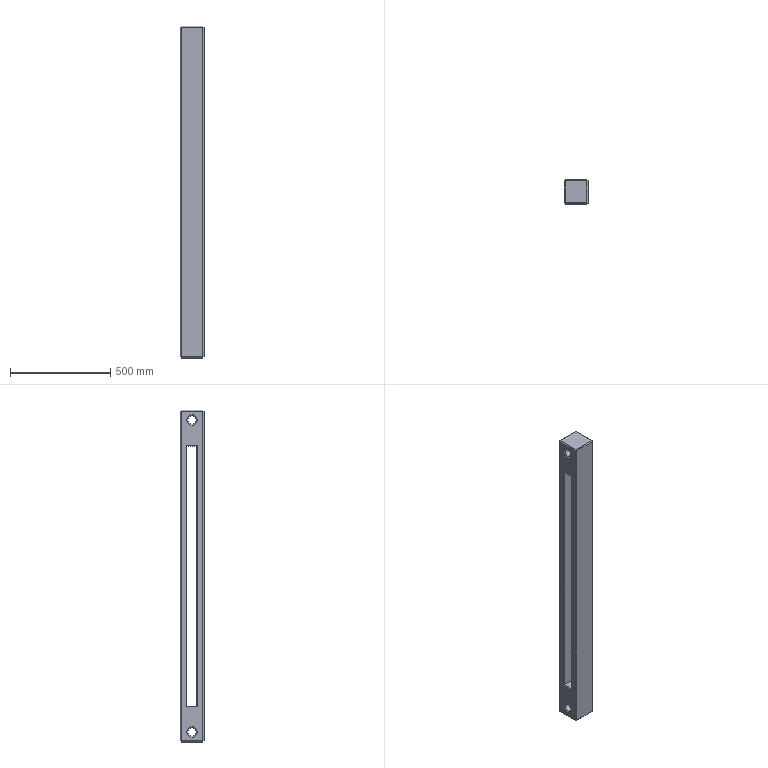Part | SolidWorks | features ICE 2, Chamfer 1, Extrusion 1 | 1 solid | 50 faces | box 120 x 120 x 1660 mm | volume 15602206 mm3 | plane 38 | cone 8 | cylinder 4 | commonest cylinder face diameters 42 x4
STEP:
#1=CARTESIAN_POINT('',(115.,0.,801.));
#2=VERTEX_POINT('',#1);
#3=CARTESIAN_POINT('',(115.,0.,759.));
#4=VERTEX_POINT('',#3);
#5=CARTESIAN_POINT('',(115.,0.,780.));
#6=DIRECTION('',(1.,0.,0.));
#7=DIRECTION('',(0.,0.,-1.));
#8=AXIS2_PLACEMENT_3D('',#5,#6,#7);
#9=CIRCLE('',#8,21.);
#10=EDGE_CURVE('',#2,#4,#9,.T.);
#11=ORIENTED_EDGE('',*,*,#10,.F.);
#12=CARTESIAN_POINT('',(120.,0.,806.));
#13=VERTEX_POINT('',#12);
#14=CARTESIAN_POINT('',(115.,0.,801.));
#15=DIRECTION('',(0.7071,0.,0.7071));
#16=VECTOR('',#15,1000.);
#17=LINE('',#14,#16);
#18=EDGE_CURVE('',#2,#13,#17,.T.);
#19=ORIENTED_EDGE('',*,*,#18,.T.);
#20=CARTESIAN_POINT('',(120.,0.,754.));
#21=VERTEX_POINT('',#20);
#22=CARTESIAN_POINT('',(120.,0.,780.));
#23=DIRECTION('',(-1.,0.,0.));
#24=DIRECTION('',(0.,0.,-1.));
#25=AXIS2_PLACEMENT_3D('',#22,#23,#24);
#26=CIRCLE('',#25,26.);
#27=EDGE_CURVE('',#21,#13,#26,.T.);
#28=ORIENTED_EDGE('',*,*,#27,.F.);
#29=CARTESIAN_POINT('',(115.,0.,759.));
#30=DIRECTION('',(0.7071,0.,-0.7071));
#31=VECTOR('',#30,1000.);
#32=LINE('',#29,#31);
#33=EDGE_CURVE('',#4,#21,#32,.T.);
#34=ORIENTED_EDGE('',*,*,#33,.F.);
#35=EDGE_LOOP('',(#11,#19,#28,#34));
#36=FACE_OUTER_BOUND('',#35,.T.);
#37=CARTESIAN_POINT('',(115.,0.,780.));
#38=DIRECTION('',(1.,0.,0.));
#39=DIRECTION('',(0.,0.,-1.));
#40=AXIS2_PLACEMENT_3D('',#37,#38,#39);
#41=CONICAL_SURFACE('',#40,21.,0.7854);
#42=ADVANCED_FACE('',(#36),#41,.F.);
#43=CARTESIAN_POINT('',(115.,0.,-759.));
#44=VERTEX_POINT('',#43);
#45=CARTESIAN_POINT('',(115.,0.,-801.));
#46=VERTEX_POINT('',#45);
#47=CARTESIAN_POINT('',(115.,0.,-780.));
#48=DIRECTION('',(1.,0.,0.));
#49=DIRECTION('',(0.,0.,-1.));
#50=AXIS2_PLACEMENT_3D('',#47,#48,#49);
#51=CIRCLE('',#50,21.);
#52=EDGE_CURVE('',#44,#46,#51,.T.);
#53=ORIENTED_EDGE('',*,*,#52,.F.);
#54=CARTESIAN_POINT('',(120.,0.,-754.));
#55=VERTEX_POINT('',#54);
#56=CARTESIAN_POINT('',(115.,0.,-759.));
#57=DIRECTION('',(0.7071,0.,0.7071));
#58=VECTOR('',#57,1000.);
#59=LINE('',#56,#58);
#60=EDGE_CURVE('',#44,#55,#59,.T.);
#61=ORIENTED_EDGE('',*,*,#60,.T.);
#62=CARTESIAN_POINT('',(120.,0.,-806.));
#63=VERTEX_POINT('',#62);
#64=CARTESIAN_POINT('',(120.,0.,-780.));
#65=DIRECTION('',(-1.,0.,0.));
#66=DIRECTION('',(0.,0.,-1.));
#67=AXIS2_PLACEMENT_3D('',#64,#65,#66);
#68=CIRCLE('',#67,26.);
#69=EDGE_CURVE('',#63,#55,#68,.T.);
#70=ORIENTED_EDGE('',*,*,#69,.F.);
#71=CARTESIAN_POINT('',(115.,0.,-801.));
#72=DIRECTION('',(0.7071,0.,-0.7071));
#73=VECTOR('',#72,1000.);
#74=LINE('',#71,#73);
#75=EDGE_CURVE('',#46,#63,#74,.T.);
#76=ORIENTED_EDGE('',*,*,#75,.F.);
#77=EDGE_LOOP('',(#53,#61,#70,#76));
#78=FACE_OUTER_BOUND('',#77,.T.);
#79=CARTESIAN_POINT('',(115.,0.,-780.));
#80=DIRECTION('',(1.,0.,0.));
#81=DIRECTION('',(0.,0.,-1.));
#82=AXIS2_PLACEMENT_3D('',#79,#80,#81);
#83=CONICAL_SURFACE('',#82,21.,0.7854);
#84=ADVANCED_FACE('',(#78),#83,.F.);
#85=CARTESIAN_POINT('',(5.,0.,759.));
#86=VERTEX_POINT('',#85);
#87=CARTESIAN_POINT('',(5.,0.,801.));
#88=VERTEX_POINT('',#87);
#89=CARTESIAN_POINT('',(5.,0.,780.));
#90=DIRECTION('',(-1.,0.,0.));
#91=DIRECTION('',(0.,0.,-1.));
#92=AXIS2_PLACEMENT_3D('',#89,#90,#91);
#93=CIRCLE('',#92,21.);
#94=EDGE_CURVE('',#86,#88,#93,.T.);
#95=ORIENTED_EDGE('',*,*,#94,.F.);
#96=CARTESIAN_POINT('',(0.,0.,754.));
#97=VERTEX_POINT('',#96);
#98=CARTESIAN_POINT('',(0.,0.,754.));
#99=DIRECTION('',(-0.7071,0.,-0.7071));
#100=VECTOR('',#99,1000.);
#101=LINE('',#98,#100);
#102=EDGE_CURVE('',#86,#97,#101,.T.);
#103=ORIENTED_EDGE('',*,*,#102,.T.);
#104=CARTESIAN_POINT('',(0.,0.,806.));
#105=VERTEX_POINT('',#104);
#106=CARTESIAN_POINT('',(0.,0.,780.));
#107=DIRECTION('',(1.,0.,0.));
#108=DIRECTION('',(0.,0.,-1.));
#109=AXIS2_PLACEMENT_3D('',#106,#107,#108);
#110=CIRCLE('',#109,26.);
#111=EDGE_CURVE('',#105,#97,#110,.T.);
#112=ORIENTED_EDGE('',*,*,#111,.F.);
#113=CARTESIAN_POINT('',(0.,0.,806.));
#114=DIRECTION('',(-0.7071,0.,0.7071));
#115=VECTOR('',#114,1000.);
#116=LINE('',#113,#115);
#117=EDGE_CURVE('',#88,#105,#116,.T.);
#118=ORIENTED_EDGE('',*,*,#117,.F.);
#119=EDGE_LOOP('',(#95,#103,#112,#118));
#120=FACE_OUTER_BOUND('',#119,.T.);
#121=CARTESIAN_POINT('',(0.,0.,780.));
#122=DIRECTION('',(-1.,0.,0.));
#123=DIRECTION('',(0.,0.,1.));
#124=AXIS2_PLACEMENT_3D('',#121,#122,#123);
#125=CONICAL_SURFACE('',#124,26.,0.7854);
#126=ADVANCED_FACE('',(#120),#125,.F.);
#127=CARTESIAN_POINT('',(5.,0.,-801.));
#128=VERTEX_POINT('',#127);
#129=CARTESIAN_POINT('',(5.,0.,-759.));
#130=VERTEX_POINT('',#129);
#131=CARTESIAN_POINT('',(5.,0.,-780.));
#132=DIRECTION('',(-1.,0.,0.));
#133=DIRECTION('',(0.,0.,-1.));
#134=AXIS2_PLACEMENT_3D('',#131,#132,#133);
#135=CIRCLE('',#134,21.);
#136=EDGE_CURVE('',#128,#130,#135,.T.);
#137=ORIENTED_EDGE('',*,*,#136,.F.);
#138=CARTESIAN_POINT('',(0.,0.,-806.));
#139=VERTEX_POINT('',#138);
#140=CARTESIAN_POINT('',(0.,0.,-806.));
#141=DIRECTION('',(-0.7071,0.,-0.7071));
#142=VECTOR('',#141,1000.);
#143=LINE('',#140,#142);
#144=EDGE_CURVE('',#128,#139,#143,.T.);
#145=ORIENTED_EDGE('',*,*,#144,.T.);
#146=CARTESIAN_POINT('',(0.,0.,-754.));
#147=VERTEX_POINT('',#146);
#148=CARTESIAN_POINT('',(0.,0.,-780.));
#149=DIRECTION('',(1.,0.,0.));
#150=DIRECTION('',(0.,0.,-1.));
#151=AXIS2_PLACEMENT_3D('',#148,#149,#150);
#152=CIRCLE('',#151,26.);
#153=EDGE_CURVE('',#147,#139,#152,.T.);
#154=ORIENTED_EDGE('',*,*,#153,.F.);
#155=CARTESIAN_POINT('',(0.,0.,-754.));
#156=DIRECTION('',(-0.7071,0.,0.7071));
#157=VECTOR('',#156,1000.);
#158=LINE('',#155,#157);
#159=EDGE_CURVE('',#130,#147,#158,.T.);
#160=ORIENTED_EDGE('',*,*,#159,.F.);
#161=EDGE_LOOP('',(#137,#145,#154,#160));
#162=FACE_OUTER_BOUND('',#161,.T.);
#163=CARTESIAN_POINT('',(0.,0.,-780.));
#164=DIRECTION('',(-1.,0.,0.));
#165=DIRECTION('',(0.,0.,1.));
#166=AXIS2_PLACEMENT_3D('',#163,#164,#165);
#167=CONICAL_SURFACE('',#166,26.,0.7854);
#168=ADVANCED_FACE('',(#162),#167,.F.);
#169=ORIENTED_EDGE('',*,*,#94,.T.);
#170=CARTESIAN_POINT('',(0.,0.,801.));
#171=DIRECTION('',(1.,0.,0.));
#172=VECTOR('',#171,1000.);
#173=LINE('',#170,#172);
#174=EDGE_CURVE('',#88,#2,#173,.T.);
#175=ORIENTED_EDGE('',*,*,#174,.T.);
#176=ORIENTED_EDGE('',*,*,#10,.T.);
#177=CARTESIAN_POINT('',(0.,0.,759.));
#178=DIRECTION('',(1.,0.,0.));
#179=VECTOR('',#178,1000.);
#180=LINE('',#177,#179);
#181=EDGE_CURVE('',#86,#4,#180,.T.);
#182=ORIENTED_EDGE('',*,*,#181,.F.);
#183=EDGE_LOOP('',(#169,#175,#176,#182));
#184=FACE_OUTER_BOUND('',#183,.T.);
#185=CARTESIAN_POINT('',(0.,0.,780.));
#186=DIRECTION('',(1.,0.,0.));
#187=DIRECTION('',(0.,0.,-1.));
#188=AXIS2_PLACEMENT_3D('',#185,#186,#187);
#189=CYLINDRICAL_SURFACE('',#188,21.);
#190=ADVANCED_FACE('',(#184),#189,.F.);
#191=ORIENTED_EDGE('',*,*,#136,.T.);
#192=CARTESIAN_POINT('',(0.,0.,-759.));
#193=DIRECTION('',(1.,0.,0.));
#194=VECTOR('',#193,1000.);
#195=LINE('',#192,#194);
#196=EDGE_CURVE('',#130,#44,#195,.T.);
#197=ORIENTED_EDGE('',*,*,#196,.T.);
#198=ORIENTED_EDGE('',*,*,#52,.T.);
#199=CARTESIAN_POINT('',(0.,0.,-801.));
#200=DIRECTION('',(1.,0.,0.));
#201=VECTOR('',#200,1000.);
#202=LINE('',#199,#201);
#203=EDGE_CURVE('',#128,#46,#202,.T.);
#204=ORIENTED_EDGE('',*,*,#203,.F.);
#205=EDGE_LOOP('',(#191,#197,#198,#204));
#206=FACE_OUTER_BOUND('',#205,.T.);
#207=CARTESIAN_POINT('',(0.,0.,-780.));
#208=DIRECTION('',(1.,0.,0.));
#209=DIRECTION('',(0.,0.,-1.));
#210=AXIS2_PLACEMENT_3D('',#207,#208,#209);
#211=CYLINDRICAL_SURFACE('',#210,21.);
#212=ADVANCED_FACE('',(#206),#211,.F.);
#213=CARTESIAN_POINT('',(115.,55.,-830.));
#214=VERTEX_POINT('',#213);
#215=CARTESIAN_POINT('',(115.,-55.,-830.));
#216=VERTEX_POINT('',#215);
#217=CARTESIAN_POINT('',(115.,-60.,-830.));
#218=DIRECTION('',(0.,-1.,0.));
#219=VECTOR('',#218,1000.);
#220=LINE('',#217,#219);
#221=EDGE_CURVE('',#214,#216,#220,.T.);
#222=ORIENTED_EDGE('',*,*,#221,.T.);
#223=CARTESIAN_POINT('',(5.,-55.,-830.));
#224=VERTEX_POINT('',#223);
#225=CARTESIAN_POINT('',(120.,-55.,-830.));
#226=DIRECTION('',(-1.,0.,0.));
#227=VECTOR('',#226,1000.);
#228=LINE('',#225,#227);
#229=EDGE_CURVE('',#216,#224,#228,.T.);
#230=ORIENTED_EDGE('',*,*,#229,.T.);
#231=CARTESIAN_POINT('',(5.,55.,-830.));
#232=VERTEX_POINT('',#231);
#233=CARTESIAN_POINT('',(5.,60.,-830.));
#234=DIRECTION('',(0.,1.,0.));
#235=VECTOR('',#234,1000.);
#236=LINE('',#233,#235);
#237=EDGE_CURVE('',#224,#232,#236,.T.);
#238=ORIENTED_EDGE('',*,*,#237,.T.);
#239=CARTESIAN_POINT('',(120.,55.,-830.));
#240=DIRECTION('',(1.,0.,0.));
#241=VECTOR('',#240,1000.);
#242=LINE('',#239,#241);
#243=EDGE_CURVE('',#232,#214,#242,.T.);
#244=ORIENTED_EDGE('',*,*,#243,.T.);
#245=EDGE_LOOP('',(#222,#230,#238,#244));
#246=FACE_OUTER_BOUND('',#245,.T.);
#247=CARTESIAN_POINT('',(120.,60.,-830.));
#248=DIRECTION('',(0.,0.,1.));
#249=DIRECTION('',(1.,0.,0.));
#250=AXIS2_PLACEMENT_3D('',#247,#248,#249);
#251=PLANE('',#250);
#252=ADVANCED_FACE('',(#246),#251,.F.);
#253=CARTESIAN_POINT('',(115.,60.,-825.));
#254=VERTEX_POINT('',#253);
#255=CARTESIAN_POINT('',(5.,60.,-825.));
#256=VERTEX_POINT('',#255);
#257=CARTESIAN_POINT('',(120.,60.,-825.));
#258=DIRECTION('',(-1.,0.,0.));
#259=VECTOR('',#258,1000.);
#260=LINE('',#257,#259);
#261=EDGE_CURVE('',#254,#256,#260,.T.);
#262=ORIENTED_EDGE('',*,*,#261,.T.);
#263=CARTESIAN_POINT('',(5.,60.,825.));
#264=VERTEX_POINT('',#263);
#265=CARTESIAN_POINT('',(5.,60.,830.));
#266=DIRECTION('',(0.,0.,1.));
#267=VECTOR('',#266,1000.);
#268=LINE('',#265,#267);
#269=EDGE_CURVE('',#256,#264,#268,.T.);
#270=ORIENTED_EDGE('',*,*,#269,.T.);
#271=CARTESIAN_POINT('',(115.,60.,825.));
#272=VERTEX_POINT('',#271);
#273=CARTESIAN_POINT('',(120.,60.,825.));
#274=DIRECTION('',(1.,0.,0.));
#275=VECTOR('',#274,1000.);
#276=LINE('',#273,#275);
#277=EDGE_CURVE('',#264,#272,#276,.T.);
#278=ORIENTED_EDGE('',*,*,#277,.T.);
#279=CARTESIAN_POINT('',(115.,60.,-830.));
#280=DIRECTION('',(0.,0.,-1.));
#281=VECTOR('',#280,1000.);
#282=LINE('',#279,#281);
#283=EDGE_CURVE('',#272,#254,#282,.T.);
#284=ORIENTED_EDGE('',*,*,#283,.T.);
#285=EDGE_LOOP('',(#262,#270,#278,#284));
#286=FACE_OUTER_BOUND('',#285,.T.);
#287=CARTESIAN_POINT('',(120.,60.,830.));
#288=DIRECTION('',(0.,-1.,0.));
#289=DIRECTION('',(0.,0.,-1.));
#290=AXIS2_PLACEMENT_3D('',#287,#288,#289);
#291=PLANE('',#290);
#292=ADVANCED_FACE('',(#286),#291,.F.);
#293=CARTESIAN_POINT('',(115.,-55.,830.));
#294=VERTEX_POINT('',#293);
#295=CARTESIAN_POINT('',(115.,55.,830.));
#296=VERTEX_POINT('',#295);
#297=CARTESIAN_POINT('',(115.,60.,830.));
#298=DIRECTION('',(0.,1.,0.));
#299=VECTOR('',#298,1000.);
#300=LINE('',#297,#299);
#301=EDGE_CURVE('',#294,#296,#300,.T.);
#302=ORIENTED_EDGE('',*,*,#301,.T.);
#303=CARTESIAN_POINT('',(5.,55.,830.));
#304=VERTEX_POINT('',#303);
#305=CARTESIAN_POINT('',(120.,55.,830.));
#306=DIRECTION('',(-1.,0.,0.));
#307=VECTOR('',#306,1000.);
#308=LINE('',#305,#307);
#309=EDGE_CURVE('',#296,#304,#308,.T.);
#310=ORIENTED_EDGE('',*,*,#309,.T.);
#311=CARTESIAN_POINT('',(5.,-55.,830.));
#312=VERTEX_POINT('',#311);
#313=CARTESIAN_POINT('',(5.,60.,830.));
#314=DIRECTION('',(0.,-1.,0.));
#315=VECTOR('',#314,1000.);
#316=LINE('',#313,#315);
#317=EDGE_CURVE('',#304,#312,#316,.T.);
#318=ORIENTED_EDGE('',*,*,#317,.T.);
#319=CARTESIAN_POINT('',(120.,-55.,830.));
#320=DIRECTION('',(1.,0.,0.));
#321=VECTOR('',#320,1000.);
#322=LINE('',#319,#321);
#323=EDGE_CURVE('',#312,#294,#322,.T.);
#324=ORIENTED_EDGE('',*,*,#323,.T.);
#325=EDGE_LOOP('',(#302,#310,#318,#324));
#326=FACE_OUTER_BOUND('',#325,.T.);
#327=CARTESIAN_POINT('',(120.,60.,830.));
#328=DIRECTION('',(0.,0.,-1.));
#329=DIRECTION('',(-1.,0.,0.));
#330=AXIS2_PLACEMENT_3D('',#327,#328,#329);
#331=PLANE('',#330);
#332=ADVANCED_FACE('',(#326),#331,.F.);
#333=CARTESIAN_POINT('',(115.,-60.,825.));
#334=VERTEX_POINT('',#333);
#335=CARTESIAN_POINT('',(5.,-60.,825.));
#336=VERTEX_POINT('',#335);
#337=CARTESIAN_POINT('',(120.,-60.,825.));
#338=DIRECTION('',(-1.,0.,0.));
#339=VECTOR('',#338,1000.);
#340=LINE('',#337,#339);
#341=EDGE_CURVE('',#334,#336,#340,.T.);
#342=ORIENTED_EDGE('',*,*,#341,.T.);
#343=CARTESIAN_POINT('',(5.,-60.,-825.));
#344=VERTEX_POINT('',#343);
#345=CARTESIAN_POINT('',(5.,-60.,830.));
#346=DIRECTION('',(0.,0.,-1.));
#347=VECTOR('',#346,1000.);
#348=LINE('',#345,#347);
#349=EDGE_CURVE('',#336,#344,#348,.T.);
#350=ORIENTED_EDGE('',*,*,#349,.T.);
#351=CARTESIAN_POINT('',(115.,-60.,-825.));
#352=VERTEX_POINT('',#351);
#353=CARTESIAN_POINT('',(120.,-60.,-825.));
#354=DIRECTION('',(1.,0.,0.));
#355=VECTOR('',#354,1000.);
#356=LINE('',#353,#355);
#357=EDGE_CURVE('',#344,#352,#356,.T.);
#358=ORIENTED_EDGE('',*,*,#357,.T.);
#359=CARTESIAN_POINT('',(115.,-60.,830.));
#360=DIRECTION('',(0.,0.,1.));
#361=VECTOR('',#360,1000.);
#362=LINE('',#359,#361);
#363=EDGE_CURVE('',#352,#334,#362,.T.);
#364=ORIENTED_EDGE('',*,*,#363,.T.);
#365=EDGE_LOOP('',(#342,#350,#358,#364));
#366=FACE_OUTER_BOUND('',#365,.T.);
#367=CARTESIAN_POINT('',(120.,-60.,830.));
#368=DIRECTION('',(0.,1.,0.));
#369=DIRECTION('',(0.,0.,1.));
#370=AXIS2_PLACEMENT_3D('',#367,#368,#369);
#371=PLANE('',#370);
#372=ADVANCED_FACE('',(#366),#371,.F.);
#373=CARTESIAN_POINT('',(120.,-30.,655.));
#374=VERTEX_POINT('',#373);
#375=CARTESIAN_POINT('',(120.,30.,655.));
#376=VERTEX_POINT('',#375);
#377=CARTESIAN_POINT('',(120.,25.,655.));
#378=DIRECTION('',(0.,1.,0.));
#379=VECTOR('',#378,1000.);
#380=LINE('',#377,#379);
#381=EDGE_CURVE('',#374,#376,#380,.T.);
#382=ORIENTED_EDGE('',*,*,#381,.T.);
#383=CARTESIAN_POINT('',(120.,30.,-655.));
#384=VERTEX_POINT('',#383);
#385=CARTESIAN_POINT('',(120.,30.,-650.));
#386=DIRECTION('',(0.,0.,-1.));
#387=VECTOR('',#386,1000.);
#388=LINE('',#385,#387);
#389=EDGE_CURVE('',#376,#384,#388,.T.);
#390=ORIENTED_EDGE('',*,*,#389,.T.);
#391=CARTESIAN_POINT('',(120.,-30.,-655.));
#392=VERTEX_POINT('',#391);
#393=CARTESIAN_POINT('',(120.,-25.,-655.));
#394=DIRECTION('',(0.,-1.,0.));
#395=VECTOR('',#394,1000.);
#396=LINE('',#393,#395);
#397=EDGE_CURVE('',#384,#392,#396,.T.);
#398=ORIENTED_EDGE('',*,*,#397,.T.);
#399=CARTESIAN_POINT('',(120.,-30.,650.));
#400=DIRECTION('',(0.,0.,1.));
#401=VECTOR('',#400,1000.);
#402=LINE('',#399,#401);
#403=EDGE_CURVE('',#392,#374,#402,.T.);
#404=ORIENTED_EDGE('',*,*,#403,.T.);
#405=EDGE_LOOP('',(#382,#390,#398,#404));
#406=FACE_BOUND('',#405,.T.);
#407=ORIENTED_EDGE('',*,*,#69,.T.);
#408=CARTESIAN_POINT('',(120.,0.,-780.));
#409=DIRECTION('',(-1.,0.,0.));
#410=DIRECTION('',(0.,0.,-1.));
#411=AXIS2_PLACEMENT_3D('',#408,#409,#410);
#412=CIRCLE('',#411,26.);
#413=EDGE_CURVE('',#55,#63,#412,.T.);
#414=ORIENTED_EDGE('',*,*,#413,.T.);
#415=EDGE_LOOP('',(#407,#414));
#416=FACE_BOUND('',#415,.T.);
#417=ORIENTED_EDGE('',*,*,#27,.T.);
#418=CARTESIAN_POINT('',(120.,0.,780.));
#419=DIRECTION('',(-1.,0.,0.));
#420=DIRECTION('',(0.,0.,-1.));
#421=AXIS2_PLACEMENT_3D('',#418,#419,#420);
#422=CIRCLE('',#421,26.);
#423=EDGE_CURVE('',#13,#21,#422,.T.);
#424=ORIENTED_EDGE('',*,*,#423,.T.);
#425=EDGE_LOOP('',(#417,#424));
#426=FACE_BOUND('',#425,.T.);
#427=CARTESIAN_POINT('',(120.,55.,825.));
#428=VERTEX_POINT('',#427);
#429=CARTESIAN_POINT('',(120.,-55.,825.));
#430=VERTEX_POINT('',#429);
#431=CARTESIAN_POINT('',(120.,-60.,825.));
#432=DIRECTION('',(0.,-1.,0.));
#433=VECTOR('',#432,1000.);
#434=LINE('',#431,#433);
#435=EDGE_CURVE('',#428,#430,#434,.T.);
#436=ORIENTED_EDGE('',*,*,#435,.T.);
#437=CARTESIAN_POINT('',(120.,-55.,-825.));
#438=VERTEX_POINT('',#437);
#439=CARTESIAN_POINT('',(120.,-55.,-830.));
#440=DIRECTION('',(0.,0.,-1.));
#441=VECTOR('',#440,1000.);
#442=LINE('',#439,#441);
#443=EDGE_CURVE('',#430,#438,#442,.T.);
#444=ORIENTED_EDGE('',*,*,#443,.T.);
#445=CARTESIAN_POINT('',(120.,55.,-825.));
#446=VERTEX_POINT('',#445);
#447=CARTESIAN_POINT('',(120.,60.,-825.));
#448=DIRECTION('',(0.,1.,0.));
#449=VECTOR('',#448,1000.);
#450=LINE('',#447,#449);
#451=EDGE_CURVE('',#438,#446,#450,.T.);
#452=ORIENTED_EDGE('',*,*,#451,.T.);
#453=CARTESIAN_POINT('',(120.,55.,830.));
#454=DIRECTION('',(0.,0.,1.));
#455=VECTOR('',#454,1000.);
#456=LINE('',#453,#455);
#457=EDGE_CURVE('',#446,#428,#456,.T.);
#458=ORIENTED_EDGE('',*,*,#457,.T.);
#459=EDGE_LOOP('',(#436,#444,#452,#458));
#460=FACE_OUTER_BOUND('',#459,.T.);
#461=CARTESIAN_POINT('',(120.,0.,0.));
#462=DIRECTION('',(1.,0.,0.));
#463=DIRECTION('',(0.,0.,-1.));
#464=AXIS2_PLACEMENT_3D('',#461,#462,#463);
#465=PLANE('',#464);
#466=ADVANCED_FACE('',(#406,#416,#426,#460),#465,.T.);
#467=CARTESIAN_POINT('',(0.,30.,-655.));
#468=VERTEX_POINT('',#467);
#469=CARTESIAN_POINT('',(0.,30.,655.));
#470=VERTEX_POINT('',#469);
#471=CARTESIAN_POINT('',(0.,30.,0.));
#472=DIRECTION('',(0.,0.,1.));
#473=VECTOR('',#472,1000.);
#474=LINE('',#471,#473);
#475=EDGE_CURVE('',#468,#470,#474,.T.);
#476=ORIENTED_EDGE('',*,*,#475,.T.);
#477=CARTESIAN_POINT('',(0.,-30.,655.));
#478=VERTEX_POINT('',#477);
#479=CARTESIAN_POINT('',(0.,0.,655.));
#480=DIRECTION('',(0.,-1.,0.));
#481=VECTOR('',#480,1000.);
#482=LINE('',#479,#481);
#483=EDGE_CURVE('',#470,#478,#482,.T.);
#484=ORIENTED_EDGE('',*,*,#483,.T.);
#485=CARTESIAN_POINT('',(0.,-30.,-655.));
#486=VERTEX_POINT('',#485);
#487=CARTESIAN_POINT('',(0.,-30.,0.));
#488=DIRECTION('',(0.,0.,-1.));
#489=VECTOR('',#488,1000.);
#490=LINE('',#487,#489);
#491=EDGE_CURVE('',#478,#486,#490,.T.);
#492=ORIENTED_EDGE('',*,*,#491,.T.);
#493=CARTESIAN_POINT('',(0.,0.,-655.));
#494=DIRECTION('',(0.,1.,0.));
#495=VECTOR('',#494,1000.);
#496=LINE('',#493,#495);
#497=EDGE_CURVE('',#486,#468,#496,.T.);
#498=ORIENTED_EDGE('',*,*,#497,.T.);
#499=EDGE_LOOP('',(#476,#484,#492,#498));
#500=FACE_BOUND('',#499,.T.);
#501=ORIENTED_EDGE('',*,*,#153,.T.);
#502=CARTESIAN_POINT('',(0.,0.,-780.));
#503=DIRECTION('',(1.,0.,0.));
#504=DIRECTION('',(0.,0.,-1.));
#505=AXIS2_PLACEMENT_3D('',#502,#503,#504);
#506=CIRCLE('',#505,26.);
#507=EDGE_CURVE('',#139,#147,#506,.T.);
#508=ORIENTED_EDGE('',*,*,#507,.T.);
#509=EDGE_LOOP('',(#501,#508));
#510=FACE_BOUND('',#509,.T.);
#511=ORIENTED_EDGE('',*,*,#111,.T.);
#512=CARTESIAN_POINT('',(0.,0.,780.));
#513=DIRECTION('',(1.,0.,0.));
#514=DIRECTION('',(0.,0.,-1.));
#515=AXIS2_PLACEMENT_3D('',#512,#513,#514);
#516=CIRCLE('',#515,26.);
#517=EDGE_CURVE('',#97,#105,#516,.T.);
#518=ORIENTED_EDGE('',*,*,#517,.T.);
#519=EDGE_LOOP('',(#511,#518));
#520=FACE_BOUND('',#519,.T.);
#521=CARTESIAN_POINT('',(0.,55.,825.));
#522=VERTEX_POINT('',#521);
#523=CARTESIAN_POINT('',(0.,55.,-825.));
#524=VERTEX_POINT('',#523);
#525=CARTESIAN_POINT('',(0.,55.,0.));
#526=DIRECTION('',(0.,0.,-1.));
#527=VECTOR('',#526,1000.);
#528=LINE('',#525,#527);
#529=EDGE_CURVE('',#522,#524,#528,.T.);
#530=ORIENTED_EDGE('',*,*,#529,.T.);
#531=CARTESIAN_POINT('',(0.,-55.,-825.));
#532=VERTEX_POINT('',#531);
#533=CARTESIAN_POINT('',(0.,0.,-825.));
#534=DIRECTION('',(0.,-1.,0.));
#535=VECTOR('',#534,1000.);
#536=LINE('',#533,#535);
#537=EDGE_CURVE('',#524,#532,#536,.T.);
#538=ORIENTED_EDGE('',*,*,#537,.T.);
#539=CARTESIAN_POINT('',(0.,-55.,825.));
#540=VERTEX_POINT('',#539);
#541=CARTESIAN_POINT('',(0.,-55.,0.));
#542=DIRECTION('',(0.,0.,1.));
#543=VECTOR('',#542,1000.);
#544=LINE('',#541,#543);
#545=EDGE_CURVE('',#532,#540,#544,.T.);
#546=ORIENTED_EDGE('',*,*,#545,.T.);
#547=CARTESIAN_POINT('',(0.,0.,825.));
#548=DIRECTION('',(0.,1.,0.));
#549=VECTOR('',#548,1000.);
#550=LINE('',#547,#549);
#551=EDGE_CURVE('',#540,#522,#550,.T.);
#552=ORIENTED_EDGE('',*,*,#551,.T.);
#553=EDGE_LOOP('',(#530,#538,#546,#552));
#554=FACE_OUTER_BOUND('',#553,.T.);
#555=CARTESIAN_POINT('',(0.,0.,0.));
#556=DIRECTION('',(1.,0.,0.));
#557=DIRECTION('',(0.,0.,-1.));
#558=AXIS2_PLACEMENT_3D('',#555,#556,#557);
#559=PLANE('',#558);
#560=ADVANCED_FACE('',(#500,#510,#520,#554),#559,.F.);
#561=CARTESIAN_POINT('',(5.,25.,-650.));
#562=VERTEX_POINT('',#561);
#563=CARTESIAN_POINT('',(115.,25.,-650.));
#564=VERTEX_POINT('',#563);
#565=CARTESIAN_POINT('',(0.,25.,-650.));
#566=DIRECTION('',(1.,0.,0.));
#567=VECTOR('',#566,1000.);
#568=LINE('',#565,#567);
#569=EDGE_CURVE('',#562,#564,#568,.T.);
#570=ORIENTED_EDGE('',*,*,#569,.F.);
#571=CARTESIAN_POINT('',(5.,-25.,-650.));
#572=VERTEX_POINT('',#571);
#573=CARTESIAN_POINT('',(5.,25.,-650.));
#574=DIRECTION('',(0.,-1.,0.));
#575=VECTOR('',#574,1000.);
#576=LINE('',#573,#575);
#577=EDGE_CURVE('',#562,#572,#576,.T.);
#578=ORIENTED_EDGE('',*,*,#577,.T.);
#579=CARTESIAN_POINT('',(115.,-25.,-650.));
#580=VERTEX_POINT('',#579);
#581=CARTESIAN_POINT('',(0.,-25.,-650.));
#582=DIRECTION('',(1.,0.,0.));
#583=VECTOR('',#582,1000.);
#584=LINE('',#581,#583);
#585=EDGE_CURVE('',#572,#580,#584,.T.);
#586=ORIENTED_EDGE('',*,*,#585,.T.);
#587=CARTESIAN_POINT('',(115.,25.,-650.));
#588=DIRECTION('',(0.,1.,0.));
#589=VECTOR('',#588,1000.);
#590=LINE('',#587,#589);
#591=EDGE_CURVE('',#580,#564,#590,.T.);
#592=ORIENTED_EDGE('',*,*,#591,.T.);
#593=EDGE_LOOP('',(#570,#578,#586,#592));
#594=FACE_OUTER_BOUND('',#593,.T.);
#595=CARTESIAN_POINT('',(0.,25.,-650.));
#596=DIRECTION('',(0.,0.,-1.));
#597=DIRECTION('',(-1.,0.,0.));
#598=AXIS2_PLACEMENT_3D('',#595,#596,#597);
#599=PLANE('',#598);
#600=ADVANCED_FACE('',(#594),#599,.F.);
#601=ORIENTED_EDGE('',*,*,#585,.F.);
#602=CARTESIAN_POINT('',(5.,-25.,650.));
#603=VERTEX_POINT('',#602);
#604=CARTESIAN_POINT('',(5.,-25.,650.));
#605=DIRECTION('',(0.,0.,1.));
#606=VECTOR('',#605,1000.);
#607=LINE('',#604,#606);
#608=EDGE_CURVE('',#572,#603,#607,.T.);
#609=ORIENTED_EDGE('',*,*,#608,.T.);
#610=CARTESIAN_POINT('',(115.,-25.,650.));
#611=VERTEX_POINT('',#610);
#612=CARTESIAN_POINT('',(0.,-25.,650.));
#613=DIRECTION('',(1.,0.,0.));
#614=VECTOR('',#613,1000.);
#615=LINE('',#612,#614);
#616=EDGE_CURVE('',#603,#611,#615,.T.);
#617=ORIENTED_EDGE('',*,*,#616,.T.);
#618=CARTESIAN_POINT('',(115.,-25.,-650.));
#619=DIRECTION('',(0.,0.,-1.));
#620=VECTOR('',#619,1000.);
#621=LINE('',#618,#620);
#622=EDGE_CURVE('',#611,#580,#621,.T.);
#623=ORIENTED_EDGE('',*,*,#622,.T.);
#624=EDGE_LOOP('',(#601,#609,#617,#623));
#625=FACE_OUTER_BOUND('',#624,.T.);
#626=CARTESIAN_POINT('',(0.,-25.,650.));
#627=DIRECTION('',(0.,-1.,0.));
#628=DIRECTION('',(0.,0.,-1.));
#629=AXIS2_PLACEMENT_3D('',#626,#627,#628);
#630=PLANE('',#629);
#631=ADVANCED_FACE('',(#625),#630,.F.);
#632=ORIENTED_EDGE('',*,*,#616,.F.);
#633=CARTESIAN_POINT('',(5.,25.,650.));
#634=VERTEX_POINT('',#633);
#635=CARTESIAN_POINT('',(5.,25.,650.));
#636=DIRECTION('',(0.,1.,0.));
#637=VECTOR('',#636,1000.);
#638=LINE('',#635,#637);
#639=EDGE_CURVE('',#603,#634,#638,.T.);
#640=ORIENTED_EDGE('',*,*,#639,.T.);
#641=CARTESIAN_POINT('',(115.,25.,650.));
#642=VERTEX_POINT('',#641);
#643=CARTESIAN_POINT('',(0.,25.,650.));
#644=DIRECTION('',(1.,0.,0.));
#645=VECTOR('',#644,1000.);
#646=LINE('',#643,#645);
#647=EDGE_CURVE('',#634,#642,#646,.T.);
#648=ORIENTED_EDGE('',*,*,#647,.T.);
#649=CARTESIAN_POINT('',(115.,-25.,650.));
#650=DIRECTION('',(0.,-1.,0.));
#651=VECTOR('',#650,1000.);
#652=LINE('',#649,#651);
#653=EDGE_CURVE('',#642,#611,#652,.T.);
#654=ORIENTED_EDGE('',*,*,#653,.T.);
#655=EDGE_LOOP('',(#632,#640,#648,#654));
#656=FACE_OUTER_BOUND('',#655,.T.);
#657=CARTESIAN_POINT('',(0.,25.,650.));
#658=DIRECTION('',(0.,0.,1.));
#659=DIRECTION('',(1.,0.,0.));
#660=AXIS2_PLACEMENT_3D('',#657,#658,#659);
#661=PLANE('',#660);
#662=ADVANCED_FACE('',(#656),#661,.F.);
#663=ORIENTED_EDGE('',*,*,#647,.F.);
#664=CARTESIAN_POINT('',(5.,25.,650.));
#665=DIRECTION('',(0.,0.,-1.));
#666=VECTOR('',#665,1000.);
#667=LINE('',#664,#666);
#668=EDGE_CURVE('',#634,#562,#667,.T.);
#669=ORIENTED_EDGE('',*,*,#668,.T.);
#670=ORIENTED_EDGE('',*,*,#569,.T.);
#671=CARTESIAN_POINT('',(115.,25.,650.));
#672=DIRECTION('',(0.,0.,1.));
#673=VECTOR('',#672,1000.);
#674=LINE('',#671,#673);
#675=EDGE_CURVE('',#564,#642,#674,.T.);
#676=ORIENTED_EDGE('',*,*,#675,.T.);
#677=EDGE_LOOP('',(#663,#669,#670,#676));
#678=FACE_OUTER_BOUND('',#677,.T.);
#679=CARTESIAN_POINT('',(0.,25.,650.));
#680=DIRECTION('',(0.,1.,0.));
#681=DIRECTION('',(0.,0.,1.));
#682=AXIS2_PLACEMENT_3D('',#679,#680,#681);
#683=PLANE('',#682);
#684=ADVANCED_FACE('',(#678),#683,.F.);
#685=ORIENTED_EDGE('',*,*,#196,.F.);
#686=CARTESIAN_POINT('',(5.,0.,-780.));
#687=DIRECTION('',(-1.,0.,0.));
#688=DIRECTION('',(0.,0.,-1.));
#689=AXIS2_PLACEMENT_3D('',#686,#687,#688);
#690=CIRCLE('',#689,21.);
#691=EDGE_CURVE('',#130,#128,#690,.T.);
#692=ORIENTED_EDGE('',*,*,#691,.T.);
#693=ORIENTED_EDGE('',*,*,#203,.T.);
#694=CARTESIAN_POINT('',(115.,0.,-780.));
#695=DIRECTION('',(1.,0.,0.));
#696=DIRECTION('',(0.,0.,-1.));
#697=AXIS2_PLACEMENT_3D('',#694,#695,#696);
#698=CIRCLE('',#697,21.);
#699=EDGE_CURVE('',#46,#44,#698,.T.);
#700=ORIENTED_EDGE('',*,*,#699,.T.);
#701=EDGE_LOOP('',(#685,#692,#693,#700));
#702=FACE_OUTER_BOUND('',#701,.T.);
#703=CARTESIAN_POINT('',(0.,0.,-780.));
#704=DIRECTION('',(1.,0.,0.));
#705=DIRECTION('',(0.,0.,-1.));
#706=AXIS2_PLACEMENT_3D('',#703,#704,#705);
#707=CYLINDRICAL_SURFACE('',#706,21.);
#708=ADVANCED_FACE('',(#702),#707,.F.);
#709=ORIENTED_EDGE('',*,*,#174,.F.);
#710=CARTESIAN_POINT('',(5.,0.,780.));
#711=DIRECTION('',(-1.,0.,0.));
#712=DIRECTION('',(0.,0.,-1.));
#713=AXIS2_PLACEMENT_3D('',#710,#711,#712);
#714=CIRCLE('',#713,21.);
#715=EDGE_CURVE('',#88,#86,#714,.T.);
#716=ORIENTED_EDGE('',*,*,#715,.T.);
#717=ORIENTED_EDGE('',*,*,#181,.T.);
#718=CARTESIAN_POINT('',(115.,0.,780.));
#719=DIRECTION('',(1.,0.,0.));
#720=DIRECTION('',(0.,0.,-1.));
#721=AXIS2_PLACEMENT_3D('',#718,#719,#720);
#722=CIRCLE('',#721,21.);
#723=EDGE_CURVE('',#4,#2,#722,.T.);
#724=ORIENTED_EDGE('',*,*,#723,.T.);
#725=EDGE_LOOP('',(#709,#716,#717,#724));
#726=FACE_OUTER_BOUND('',#725,.T.);
#727=CARTESIAN_POINT('',(0.,0.,780.));
#728=DIRECTION('',(1.,0.,0.));
#729=DIRECTION('',(0.,0.,-1.));
#730=AXIS2_PLACEMENT_3D('',#727,#728,#729);
#731=CYLINDRICAL_SURFACE('',#730,21.);
#732=ADVANCED_FACE('',(#726),#731,.F.);
#733=CARTESIAN_POINT('',(10.,-20.,-645.));
#734=DIRECTION('',(-0.5774,-0.5774,-0.5774));
#735=VECTOR('',#734,1000.);
#736=LINE('',#733,#735);
#737=EDGE_CURVE('',#572,#486,#736,.T.);
#738=ORIENTED_EDGE('',*,*,#737,.F.);
#739=ORIENTED_EDGE('',*,*,#577,.F.);
#740=CARTESIAN_POINT('',(218.333,-188.333,-436.667));
#741=DIRECTION('',(0.5774,-0.5774,0.5774));
#742=VECTOR('',#741,1000.);
#743=LINE('',#740,#742);
#744=EDGE_CURVE('',#468,#562,#743,.T.);
#745=ORIENTED_EDGE('',*,*,#744,.F.);
#746=ORIENTED_EDGE('',*,*,#497,.F.);
#747=EDGE_LOOP('',(#738,#739,#745,#746));
#748=FACE_OUTER_BOUND('',#747,.T.);
#749=CARTESIAN_POINT('',(0.,0.,-655.));
#750=DIRECTION('',(0.7071,0.,-0.7071));
#751=DIRECTION('',(0.,1.,0.));
#752=AXIS2_PLACEMENT_3D('',#749,#750,#751);
#753=PLANE('',#752);
#754=ADVANCED_FACE('',(#748),#753,.F.);
#755=ORIENTED_EDGE('',*,*,#744,.T.);
#756=ORIENTED_EDGE('',*,*,#668,.F.);
#757=CARTESIAN_POINT('',(10.,20.,645.));
#758=DIRECTION('',(0.5774,-0.5774,-0.5774));
#759=VECTOR('',#758,1000.);
#760=LINE('',#757,#759);
#761=EDGE_CURVE('',#470,#634,#760,.T.);
#762=ORIENTED_EDGE('',*,*,#761,.F.);
#763=ORIENTED_EDGE('',*,*,#475,.F.);
#764=EDGE_LOOP('',(#755,#756,#762,#763));
#765=FACE_OUTER_BOUND('',#764,.T.);
#766=CARTESIAN_POINT('',(0.,30.,0.));
#767=DIRECTION('',(0.7071,0.7071,0.));
#768=DIRECTION('',(0.,0.,1.));
#769=AXIS2_PLACEMENT_3D('',#766,#767,#768);
#770=PLANE('',#769);
#771=ADVANCED_FACE('',(#765),#770,.F.);
#772=ORIENTED_EDGE('',*,*,#737,.T.);
#773=ORIENTED_EDGE('',*,*,#491,.F.);
#774=CARTESIAN_POINT('',(10.,-20.,645.));
#775=DIRECTION('',(-0.5774,-0.5774,0.5774));
#776=VECTOR('',#775,1000.);
#777=LINE('',#774,#776);
#778=EDGE_CURVE('',#603,#478,#777,.T.);
#779=ORIENTED_EDGE('',*,*,#778,.F.);
#780=ORIENTED_EDGE('',*,*,#608,.F.);
#781=EDGE_LOOP('',(#772,#773,#779,#780));
#782=FACE_OUTER_BOUND('',#781,.T.);
#783=CARTESIAN_POINT('',(0.,-30.,0.));
#784=DIRECTION('',(0.7071,-0.7071,0.));
#785=DIRECTION('',(0.,0.,-1.));
#786=AXIS2_PLACEMENT_3D('',#783,#784,#785);
#787=PLANE('',#786);
#788=ADVANCED_FACE('',(#782),#787,.F.);
#789=ORIENTED_EDGE('',*,*,#761,.T.);
#790=ORIENTED_EDGE('',*,*,#639,.F.);
#791=ORIENTED_EDGE('',*,*,#778,.T.);
#792=ORIENTED_EDGE('',*,*,#483,.F.);
#793=EDGE_LOOP('',(#789,#790,#791,#792));
#794=FACE_OUTER_BOUND('',#793,.T.);
#795=CARTESIAN_POINT('',(0.,0.,655.));
#796=DIRECTION('',(0.7071,0.,0.7071));
#797=DIRECTION('',(0.,-1.,0.));
#798=AXIS2_PLACEMENT_3D('',#795,#796,#797);
#799=PLANE('',#798);
#800=ADVANCED_FACE('',(#794),#799,.F.);
#801=ORIENTED_EDGE('',*,*,#144,.F.);
#802=ORIENTED_EDGE('',*,*,#691,.F.);
#803=ORIENTED_EDGE('',*,*,#159,.T.);
#804=ORIENTED_EDGE('',*,*,#507,.F.);
#805=EDGE_LOOP('',(#801,#802,#803,#804));
#806=FACE_OUTER_BOUND('',#805,.T.);
#807=CARTESIAN_POINT('',(0.,0.,-780.));
#808=DIRECTION('',(-1.,0.,0.));
#809=DIRECTION('',(0.,0.,1.));
#810=AXIS2_PLACEMENT_3D('',#807,#808,#809);
#811=CONICAL_SURFACE('',#810,26.,0.7854);
#812=ADVANCED_FACE('',(#806),#811,.F.);
#813=ORIENTED_EDGE('',*,*,#102,.F.);
#814=ORIENTED_EDGE('',*,*,#715,.F.);
#815=ORIENTED_EDGE('',*,*,#117,.T.);
#816=ORIENTED_EDGE('',*,*,#517,.F.);
#817=EDGE_LOOP('',(#813,#814,#815,#816));
#818=FACE_OUTER_BOUND('',#817,.T.);
#819=CARTESIAN_POINT('',(0.,0.,780.));
#820=DIRECTION('',(-1.,0.,0.));
#821=DIRECTION('',(0.,0.,1.));
#822=AXIS2_PLACEMENT_3D('',#819,#820,#821);
#823=CONICAL_SURFACE('',#822,26.,0.7854);
#824=ADVANCED_FACE('',(#818),#823,.F.);
#825=CARTESIAN_POINT('',(98.333,-8.333,633.333));
#826=DIRECTION('',(-0.5774,0.5774,-0.5774));
#827=VECTOR('',#826,1000.);
#828=LINE('',#825,#827);
#829=EDGE_CURVE('',#374,#611,#828,.T.);
#830=ORIENTED_EDGE('',*,*,#829,.F.);
#831=ORIENTED_EDGE('',*,*,#403,.F.);
#832=CARTESIAN_POINT('',(-318.333,408.333,-216.667));
#833=DIRECTION('',(0.5774,-0.5774,-0.5774));
#834=VECTOR('',#833,1000.);
#835=LINE('',#832,#834);
#836=EDGE_CURVE('',#580,#392,#835,.T.);
#837=ORIENTED_EDGE('',*,*,#836,.F.);
#838=ORIENTED_EDGE('',*,*,#622,.F.);
#839=EDGE_LOOP('',(#830,#831,#837,#838));
#840=FACE_OUTER_BOUND('',#839,.T.);
#841=CARTESIAN_POINT('',(115.,-25.,650.));
#842=DIRECTION('',(0.7071,0.7071,0.));
#843=DIRECTION('',(0.,0.,1.));
#844=AXIS2_PLACEMENT_3D('',#841,#842,#843);
#845=PLANE('',#844);
#846=ADVANCED_FACE('',(#840),#845,.T.);
#847=ORIENTED_EDGE('',*,*,#836,.T.);
#848=ORIENTED_EDGE('',*,*,#397,.F.);
#849=CARTESIAN_POINT('',(-318.333,-408.333,-216.667));
#850=DIRECTION('',(0.5774,0.5774,-0.5774));
#851=VECTOR('',#850,1000.);
#852=LINE('',#849,#851);
#853=EDGE_CURVE('',#564,#384,#852,.T.);
#854=ORIENTED_EDGE('',*,*,#853,.F.);
#855=ORIENTED_EDGE('',*,*,#591,.F.);
#856=EDGE_LOOP('',(#847,#848,#854,#855));
#857=FACE_OUTER_BOUND('',#856,.T.);
#858=CARTESIAN_POINT('',(115.,25.,-650.));
#859=DIRECTION('',(0.7071,0.,0.7071));
#860=DIRECTION('',(0.,-1.,0.));
#861=AXIS2_PLACEMENT_3D('',#858,#859,#860);
#862=PLANE('',#861);
#863=ADVANCED_FACE('',(#857),#862,.T.);
#864=ORIENTED_EDGE('',*,*,#829,.T.);
#865=ORIENTED_EDGE('',*,*,#653,.F.);
#866=CARTESIAN_POINT('',(115.,25.,650.));
#867=DIRECTION('',(-0.5774,-0.5774,-0.5774));
#868=VECTOR('',#867,1000.);
#869=LINE('',#866,#868);
#870=EDGE_CURVE('',#376,#642,#869,.T.);
#871=ORIENTED_EDGE('',*,*,#870,.F.);
#872=ORIENTED_EDGE('',*,*,#381,.F.);
#873=EDGE_LOOP('',(#864,#865,#871,#872));
#874=FACE_OUTER_BOUND('',#873,.T.);
#875=CARTESIAN_POINT('',(115.,25.,650.));
#876=DIRECTION('',(0.7071,0.,-0.7071));
#877=DIRECTION('',(0.,1.,0.));
#878=AXIS2_PLACEMENT_3D('',#875,#876,#877);
#879=PLANE('',#878);
#880=ADVANCED_FACE('',(#874),#879,.T.);
#881=ORIENTED_EDGE('',*,*,#853,.T.);
#882=ORIENTED_EDGE('',*,*,#389,.F.);
#883=ORIENTED_EDGE('',*,*,#870,.T.);
#884=ORIENTED_EDGE('',*,*,#675,.F.);
#885=EDGE_LOOP('',(#881,#882,#883,#884));
#886=FACE_OUTER_BOUND('',#885,.T.);
#887=CARTESIAN_POINT('',(115.,25.,650.));
#888=DIRECTION('',(0.7071,-0.7071,0.));
#889=DIRECTION('',(0.,0.,-1.));
#890=AXIS2_PLACEMENT_3D('',#887,#888,#889);
#891=PLANE('',#890);
#892=ADVANCED_FACE('',(#886),#891,.T.);
#893=ORIENTED_EDGE('',*,*,#60,.F.);
#894=ORIENTED_EDGE('',*,*,#699,.F.);
#895=ORIENTED_EDGE('',*,*,#75,.T.);
#896=ORIENTED_EDGE('',*,*,#413,.F.);
#897=EDGE_LOOP('',(#893,#894,#895,#896));
#898=FACE_OUTER_BOUND('',#897,.T.);
#899=CARTESIAN_POINT('',(115.,0.,-780.));
#900=DIRECTION('',(1.,0.,0.));
#901=DIRECTION('',(0.,0.,-1.));
#902=AXIS2_PLACEMENT_3D('',#899,#900,#901);
#903=CONICAL_SURFACE('',#902,21.,0.7854);
#904=ADVANCED_FACE('',(#898),#903,.F.);
#905=ORIENTED_EDGE('',*,*,#18,.F.);
#906=ORIENTED_EDGE('',*,*,#723,.F.);
#907=ORIENTED_EDGE('',*,*,#33,.T.);
#908=ORIENTED_EDGE('',*,*,#423,.F.);
#909=EDGE_LOOP('',(#905,#906,#907,#908));
#910=FACE_OUTER_BOUND('',#909,.T.);
#911=CARTESIAN_POINT('',(115.,0.,780.));
#912=DIRECTION('',(1.,0.,0.));
#913=DIRECTION('',(0.,0.,-1.));
#914=AXIS2_PLACEMENT_3D('',#911,#912,#913);
#915=CONICAL_SURFACE('',#914,21.,0.7854);
#916=ADVANCED_FACE('',(#910),#915,.F.);
#917=CARTESIAN_POINT('',(115.,-60.,-825.));
#918=DIRECTION('',(-0.7071,-0.7071,0.));
#919=VECTOR('',#918,1000.);
#920=LINE('',#917,#919);
#921=EDGE_CURVE('',#438,#352,#920,.T.);
#922=ORIENTED_EDGE('',*,*,#921,.F.);
#923=ORIENTED_EDGE('',*,*,#443,.F.);
#924=CARTESIAN_POINT('',(115.,-60.,825.));
#925=DIRECTION('',(0.7071,0.7071,0.));
#926=VECTOR('',#925,1000.);
#927=LINE('',#924,#926);
#928=EDGE_CURVE('',#334,#430,#927,.T.);
#929=ORIENTED_EDGE('',*,*,#928,.F.);
#930=ORIENTED_EDGE('',*,*,#363,.F.);
#931=EDGE_LOOP('',(#922,#923,#929,#930));
#932=FACE_OUTER_BOUND('',#931,.T.);
#933=CARTESIAN_POINT('',(120.,-55.,0.));
#934=DIRECTION('',(0.7071,-0.7071,0.));
#935=DIRECTION('',(0.,0.,1.));
#936=AXIS2_PLACEMENT_3D('',#933,#934,#935);
#937=PLANE('',#936);
#938=ADVANCED_FACE('',(#932),#937,.T.);
#939=CARTESIAN_POINT('',(117.5,-55.,-827.5));
#940=DIRECTION('',(-0.7071,0.,-0.7071));
#941=VECTOR('',#940,1000.);
#942=LINE('',#939,#941);
#943=EDGE_CURVE('',#438,#216,#942,.T.);
#944=ORIENTED_EDGE('',*,*,#943,.F.);
#945=ORIENTED_EDGE('',*,*,#921,.T.);
#946=CARTESIAN_POINT('',(115.,-60.,-825.));
#947=DIRECTION('',(0.,-0.7071,0.7071));
#948=VECTOR('',#947,1000.);
#949=LINE('',#946,#948);
#950=EDGE_CURVE('',#216,#352,#949,.T.);
#951=ORIENTED_EDGE('',*,*,#950,.F.);
#952=EDGE_LOOP('',(#944,#945,#951));
#953=FACE_OUTER_BOUND('',#952,.T.);
#954=CARTESIAN_POINT('',(115.,-60.,-825.));
#955=DIRECTION('',(0.5774,-0.5774,-0.5774));
#956=DIRECTION('',(-0.7071,0.,-0.7071));
#957=AXIS2_PLACEMENT_3D('',#954,#955,#956);
#958=PLANE('',#957);
#959=ADVANCED_FACE('',(#953),#958,.T.);
#960=CARTESIAN_POINT('',(115.,-60.,825.));
#961=DIRECTION('',(0.,0.7071,0.7071));
#962=VECTOR('',#961,1000.);
#963=LINE('',#960,#962);
#964=EDGE_CURVE('',#334,#294,#963,.T.);
#965=ORIENTED_EDGE('',*,*,#964,.F.);
#966=ORIENTED_EDGE('',*,*,#928,.T.);
#967=CARTESIAN_POINT('',(117.5,-55.,827.5));
#968=DIRECTION('',(0.7071,0.,-0.7071));
#969=VECTOR('',#968,1000.);
#970=LINE('',#967,#969);
#971=EDGE_CURVE('',#294,#430,#970,.T.);
#972=ORIENTED_EDGE('',*,*,#971,.F.);
#973=EDGE_LOOP('',(#965,#966,#972));
#974=FACE_OUTER_BOUND('',#973,.T.);
#975=CARTESIAN_POINT('',(115.,-60.,825.));
#976=DIRECTION('',(0.5774,-0.5774,0.5774));
#977=DIRECTION('',(0.7071,0.,-0.7071));
#978=AXIS2_PLACEMENT_3D('',#975,#976,#977);
#979=PLANE('',#978);
#980=ADVANCED_FACE('',(#974),#979,.T.);
#981=ORIENTED_EDGE('',*,*,#950,.T.);
#982=ORIENTED_EDGE('',*,*,#357,.F.);
#983=CARTESIAN_POINT('',(5.,-60.,-825.));
#984=DIRECTION('',(0.,-0.7071,0.7071));
#985=VECTOR('',#984,1000.);
#986=LINE('',#983,#985);
#987=EDGE_CURVE('',#224,#344,#986,.T.);
#988=ORIENTED_EDGE('',*,*,#987,.F.);
#989=ORIENTED_EDGE('',*,*,#229,.F.);
#990=EDGE_LOOP('',(#981,#982,#988,#989));
#991=FACE_OUTER_BOUND('',#990,.T.);
#992=CARTESIAN_POINT('',(120.,-55.,-830.));
#993=DIRECTION('',(0.,0.7071,0.7071));
#994=DIRECTION('',(-1.,0.,0.));
#995=AXIS2_PLACEMENT_3D('',#992,#993,#994);
#996=PLANE('',#995);
#997=ADVANCED_FACE('',(#991),#996,.F.);
#998=ORIENTED_EDGE('',*,*,#943,.T.);
#999=ORIENTED_EDGE('',*,*,#221,.F.);
#1000=CARTESIAN_POINT('',(115.,55.,-830.));
#1001=DIRECTION('',(-0.7071,0.,-0.7071));
#1002=VECTOR('',#1001,1000.);
#1003=LINE('',#1000,#1002);
#1004=EDGE_CURVE('',#446,#214,#1003,.T.);
#1005=ORIENTED_EDGE('',*,*,#1004,.F.);
#1006=ORIENTED_EDGE('',*,*,#451,.F.);
#1007=EDGE_LOOP('',(#998,#999,#1005,#1006));
#1008=FACE_OUTER_BOUND('',#1007,.T.);
#1009=CARTESIAN_POINT('',(120.,0.,-825.));
#1010=DIRECTION('',(0.7071,0.,-0.7071));
#1011=DIRECTION('',(0.,-1.,0.));
#1012=AXIS2_PLACEMENT_3D('',#1009,#1010,#1011);
#1013=PLANE('',#1012);
#1014=ADVANCED_FACE('',(#1008),#1013,.T.);
#1015=CARTESIAN_POINT('',(120.,55.,825.));
#1016=DIRECTION('',(-0.7071,0.7071,0.));
#1017=VECTOR('',#1016,1000.);
#1018=LINE('',#1015,#1017);
#1019=EDGE_CURVE('',#428,#272,#1018,.T.);
#1020=ORIENTED_EDGE('',*,*,#1019,.F.);
#1021=ORIENTED_EDGE('',*,*,#457,.F.);
#1022=CARTESIAN_POINT('',(117.5,57.5,-825.));
#1023=DIRECTION('',(0.7071,-0.7071,0.));
#1024=VECTOR('',#1023,1000.);
#1025=LINE('',#1022,#1024);
#1026=EDGE_CURVE('',#254,#446,#1025,.T.);
#1027=ORIENTED_EDGE('',*,*,#1026,.F.);
#1028=ORIENTED_EDGE('',*,*,#283,.F.);
#1029=EDGE_LOOP('',(#1020,#1021,#1027,#1028));
#1030=FACE_OUTER_BOUND('',#1029,.T.);
#1031=CARTESIAN_POINT('',(120.,55.,0.));
#1032=DIRECTION('',(0.7071,0.7071,0.));
#1033=DIRECTION('',(0.,0.,-1.));
#1034=AXIS2_PLACEMENT_3D('',#1031,#1032,#1033);
#1035=PLANE('',#1034);
#1036=ADVANCED_FACE('',(#1030),#1035,.T.);
#1037=ORIENTED_EDGE('',*,*,#971,.T.);
#1038=ORIENTED_EDGE('',*,*,#435,.F.);
#1039=CARTESIAN_POINT('',(120.,55.,825.));
#1040=DIRECTION('',(0.7071,0.,-0.7071));
#1041=VECTOR('',#1040,1000.);
#1042=LINE('',#1039,#1041);
#1043=EDGE_CURVE('',#296,#428,#1042,.T.);
#1044=ORIENTED_EDGE('',*,*,#1043,.F.);
#1045=ORIENTED_EDGE('',*,*,#301,.F.);
#1046=EDGE_LOOP('',(#1037,#1038,#1044,#1045));
#1047=FACE_OUTER_BOUND('',#1046,.T.);
#1048=CARTESIAN_POINT('',(120.,0.,825.));
#1049=DIRECTION('',(0.7071,0.,0.7071));
#1050=DIRECTION('',(0.,1.,0.));
#1051=AXIS2_PLACEMENT_3D('',#1048,#1049,#1050);
#1052=PLANE('',#1051);
#1053=ADVANCED_FACE('',(#1047),#1052,.T.);
#1054=ORIENTED_EDGE('',*,*,#964,.T.);
#1055=ORIENTED_EDGE('',*,*,#323,.F.);
#1056=CARTESIAN_POINT('',(5.,-57.5,827.5));
#1057=DIRECTION('',(0.,0.7071,0.7071));
#1058=VECTOR('',#1057,1000.);
#1059=LINE('',#1056,#1058);
#1060=EDGE_CURVE('',#336,#312,#1059,.T.);
#1061=ORIENTED_EDGE('',*,*,#1060,.F.);
#1062=ORIENTED_EDGE('',*,*,#341,.F.);
#1063=EDGE_LOOP('',(#1054,#1055,#1061,#1062));
#1064=FACE_OUTER_BOUND('',#1063,.T.);
#1065=CARTESIAN_POINT('',(120.,-60.,825.));
#1066=DIRECTION('',(0.,0.7071,-0.7071));
#1067=DIRECTION('',(-1.,0.,0.));
#1068=AXIS2_PLACEMENT_3D('',#1065,#1066,#1067);
#1069=PLANE('',#1068);
#1070=ADVANCED_FACE('',(#1064),#1069,.F.);
#1071=CARTESIAN_POINT('',(5.,-60.,-825.));
#1072=DIRECTION('',(-0.7071,0.7071,0.));
#1073=VECTOR('',#1072,1000.);
#1074=LINE('',#1071,#1073);
#1075=EDGE_CURVE('',#344,#532,#1074,.T.);
#1076=ORIENTED_EDGE('',*,*,#1075,.F.);
#1077=ORIENTED_EDGE('',*,*,#349,.F.);
#1078=CARTESIAN_POINT('',(0.,-55.,825.));
#1079=DIRECTION('',(0.7071,-0.7071,0.));
#1080=VECTOR('',#1079,1000.);
#1081=LINE('',#1078,#1080);
#1082=EDGE_CURVE('',#540,#336,#1081,.T.);
#1083=ORIENTED_EDGE('',*,*,#1082,.F.);
#1084=ORIENTED_EDGE('',*,*,#545,.F.);
#1085=EDGE_LOOP('',(#1076,#1077,#1083,#1084));
#1086=FACE_OUTER_BOUND('',#1085,.T.);
#1087=CARTESIAN_POINT('',(5.,-60.,830.));
#1088=DIRECTION('',(0.7071,0.7071,0.));
#1089=DIRECTION('',(0.,0.,-1.));
#1090=AXIS2_PLACEMENT_3D('',#1087,#1088,#1089);
#1091=PLANE('',#1090);
#1092=ADVANCED_FACE('',(#1086),#1091,.F.);
#1093=ORIENTED_EDGE('',*,*,#987,.T.);
#1094=ORIENTED_EDGE('',*,*,#1075,.T.);
#1095=CARTESIAN_POINT('',(2.5,-55.,-827.5));
#1096=DIRECTION('',(-0.7071,0.,0.7071));
#1097=VECTOR('',#1096,1000.);
#1098=LINE('',#1095,#1097);
#1099=EDGE_CURVE('',#224,#532,#1098,.T.);
#1100=ORIENTED_EDGE('',*,*,#1099,.F.);
#1101=EDGE_LOOP('',(#1093,#1094,#1100));
#1102=FACE_OUTER_BOUND('',#1101,.T.);
#1103=CARTESIAN_POINT('',(5.,-60.,-825.));
#1104=DIRECTION('',(-0.5774,-0.5774,-0.5774));
#1105=DIRECTION('',(-0.7071,0.,0.7071));
#1106=AXIS2_PLACEMENT_3D('',#1103,#1104,#1105);
#1107=PLANE('',#1106);
#1108=ADVANCED_FACE('',(#1102),#1107,.T.);
#1109=ORIENTED_EDGE('',*,*,#1026,.T.);
#1110=ORIENTED_EDGE('',*,*,#1004,.T.);
#1111=CARTESIAN_POINT('',(115.,55.,-830.));
#1112=DIRECTION('',(0.,-0.7071,-0.7071));
#1113=VECTOR('',#1112,1000.);
#1114=LINE('',#1111,#1113);
#1115=EDGE_CURVE('',#254,#214,#1114,.T.);
#1116=ORIENTED_EDGE('',*,*,#1115,.F.);
#1117=EDGE_LOOP('',(#1109,#1110,#1116));
#1118=FACE_OUTER_BOUND('',#1117,.T.);
#1119=CARTESIAN_POINT('',(115.,55.,-830.));
#1120=DIRECTION('',(0.5774,0.5774,-0.5774));
#1121=DIRECTION('',(-0.7071,0.,-0.7071));
#1122=AXIS2_PLACEMENT_3D('',#1119,#1120,#1121);
#1123=PLANE('',#1122);
#1124=ADVANCED_FACE('',(#1118),#1123,.T.);
#1125=ORIENTED_EDGE('',*,*,#1043,.T.);
#1126=ORIENTED_EDGE('',*,*,#1019,.T.);
#1127=CARTESIAN_POINT('',(115.,57.5,827.5));
#1128=DIRECTION('',(0.,0.7071,-0.7071));
#1129=VECTOR('',#1128,1000.);
#1130=LINE('',#1127,#1129);
#1131=EDGE_CURVE('',#296,#272,#1130,.T.);
#1132=ORIENTED_EDGE('',*,*,#1131,.F.);
#1133=EDGE_LOOP('',(#1125,#1126,#1132));
#1134=FACE_OUTER_BOUND('',#1133,.T.);
#1135=CARTESIAN_POINT('',(120.,55.,825.));
#1136=DIRECTION('',(0.5774,0.5774,0.5774));
#1137=DIRECTION('',(0.7071,0.,-0.7071));
#1138=AXIS2_PLACEMENT_3D('',#1135,#1136,#1137);
#1139=PLANE('',#1138);
#1140=ADVANCED_FACE('',(#1134),#1139,.T.);
#1141=ORIENTED_EDGE('',*,*,#1082,.T.);
#1142=ORIENTED_EDGE('',*,*,#1060,.T.);
#1143=CARTESIAN_POINT('',(0.,-55.,825.));
#1144=DIRECTION('',(0.7071,0.,0.7071));
#1145=VECTOR('',#1144,1000.);
#1146=LINE('',#1143,#1145);
#1147=EDGE_CURVE('',#540,#312,#1146,.T.);
#1148=ORIENTED_EDGE('',*,*,#1147,.F.);
#1149=EDGE_LOOP('',(#1141,#1142,#1148));
#1150=FACE_OUTER_BOUND('',#1149,.T.);
#1151=CARTESIAN_POINT('',(0.,-55.,825.));
#1152=DIRECTION('',(-0.5774,-0.5774,0.5774));
#1153=DIRECTION('',(0.7071,0.,0.7071));
#1154=AXIS2_PLACEMENT_3D('',#1151,#1152,#1153);
#1155=PLANE('',#1154);
#1156=ADVANCED_FACE('',(#1150),#1155,.T.);
#1157=ORIENTED_EDGE('',*,*,#1099,.T.);
#1158=ORIENTED_EDGE('',*,*,#537,.F.);
#1159=CARTESIAN_POINT('',(0.,55.,-825.));
#1160=DIRECTION('',(-0.7071,0.,0.7071));
#1161=VECTOR('',#1160,1000.);
#1162=LINE('',#1159,#1161);
#1163=EDGE_CURVE('',#232,#524,#1162,.T.);
#1164=ORIENTED_EDGE('',*,*,#1163,.F.);
#1165=ORIENTED_EDGE('',*,*,#237,.F.);
#1166=EDGE_LOOP('',(#1157,#1158,#1164,#1165));
#1167=FACE_OUTER_BOUND('',#1166,.T.);
#1168=CARTESIAN_POINT('',(5.,60.,-830.));
#1169=DIRECTION('',(0.7071,0.,0.7071));
#1170=DIRECTION('',(0.,1.,0.));
#1171=AXIS2_PLACEMENT_3D('',#1168,#1169,#1170);
#1172=PLANE('',#1171);
#1173=ADVANCED_FACE('',(#1167),#1172,.F.);
#1174=ORIENTED_EDGE('',*,*,#1115,.T.);
#1175=ORIENTED_EDGE('',*,*,#243,.F.);
#1176=CARTESIAN_POINT('',(5.,57.5,-827.5));
#1177=DIRECTION('',(0.,-0.7071,-0.7071));
#1178=VECTOR('',#1177,1000.);
#1179=LINE('',#1176,#1178);
#1180=EDGE_CURVE('',#256,#232,#1179,.T.);
#1181=ORIENTED_EDGE('',*,*,#1180,.F.);
#1182=ORIENTED_EDGE('',*,*,#261,.F.);
#1183=EDGE_LOOP('',(#1174,#1175,#1181,#1182));
#1184=FACE_OUTER_BOUND('',#1183,.T.);
#1185=CARTESIAN_POINT('',(120.,60.,-825.));
#1186=DIRECTION('',(0.,-0.7071,0.7071));
#1187=DIRECTION('',(-1.,0.,0.));
#1188=AXIS2_PLACEMENT_3D('',#1185,#1186,#1187);
#1189=PLANE('',#1188);
#1190=ADVANCED_FACE('',(#1184),#1189,.F.);
#1191=ORIENTED_EDGE('',*,*,#1131,.T.);
#1192=ORIENTED_EDGE('',*,*,#277,.F.);
#1193=CARTESIAN_POINT('',(5.,60.,825.));
#1194=DIRECTION('',(0.,0.7071,-0.7071));
#1195=VECTOR('',#1194,1000.);
#1196=LINE('',#1193,#1195);
#1197=EDGE_CURVE('',#304,#264,#1196,.T.);
#1198=ORIENTED_EDGE('',*,*,#1197,.F.);
#1199=ORIENTED_EDGE('',*,*,#309,.F.);
#1200=EDGE_LOOP('',(#1191,#1192,#1198,#1199));
#1201=FACE_OUTER_BOUND('',#1200,.T.);
#1202=CARTESIAN_POINT('',(120.,55.,830.));
#1203=DIRECTION('',(0.,-0.7071,-0.7071));
#1204=DIRECTION('',(-1.,0.,0.));
#1205=AXIS2_PLACEMENT_3D('',#1202,#1203,#1204);
#1206=PLANE('',#1205);
#1207=ADVANCED_FACE('',(#1201),#1206,.F.);
#1208=ORIENTED_EDGE('',*,*,#1147,.T.);
#1209=ORIENTED_EDGE('',*,*,#317,.F.);
#1210=CARTESIAN_POINT('',(2.5,55.,827.5));
#1211=DIRECTION('',(0.7071,0.,0.7071));
#1212=VECTOR('',#1211,1000.);
#1213=LINE('',#1210,#1212);
#1214=EDGE_CURVE('',#522,#304,#1213,.T.);
#1215=ORIENTED_EDGE('',*,*,#1214,.F.);
#1216=ORIENTED_EDGE('',*,*,#551,.F.);
#1217=EDGE_LOOP('',(#1208,#1209,#1215,#1216));
#1218=FACE_OUTER_BOUND('',#1217,.T.);
#1219=CARTESIAN_POINT('',(5.,60.,830.));
#1220=DIRECTION('',(0.7071,0.,-0.7071));
#1221=DIRECTION('',(0.,-1.,0.));
#1222=AXIS2_PLACEMENT_3D('',#1219,#1220,#1221);
#1223=PLANE('',#1222);
#1224=ADVANCED_FACE('',(#1218),#1223,.F.);
#1225=ORIENTED_EDGE('',*,*,#1180,.T.);
#1226=ORIENTED_EDGE('',*,*,#1163,.T.);
#1227=CARTESIAN_POINT('',(0.,55.,-825.));
#1228=DIRECTION('',(-0.7071,-0.7071,0.));
#1229=VECTOR('',#1228,1000.);
#1230=LINE('',#1227,#1229);
#1231=EDGE_CURVE('',#256,#524,#1230,.T.);
#1232=ORIENTED_EDGE('',*,*,#1231,.F.);
#1233=EDGE_LOOP('',(#1225,#1226,#1232));
#1234=FACE_OUTER_BOUND('',#1233,.T.);
#1235=CARTESIAN_POINT('',(0.,55.,-825.));
#1236=DIRECTION('',(-0.5774,0.5774,-0.5774));
#1237=DIRECTION('',(-0.7071,0.,0.7071));
#1238=AXIS2_PLACEMENT_3D('',#1235,#1236,#1237);
#1239=PLANE('',#1238);
#1240=ADVANCED_FACE('',(#1234),#1239,.T.);
#1241=ORIENTED_EDGE('',*,*,#1214,.T.);
#1242=ORIENTED_EDGE('',*,*,#1197,.T.);
#1243=CARTESIAN_POINT('',(5.,60.,825.));
#1244=DIRECTION('',(0.7071,0.7071,0.));
#1245=VECTOR('',#1244,1000.);
#1246=LINE('',#1243,#1245);
#1247=EDGE_CURVE('',#522,#264,#1246,.T.);
#1248=ORIENTED_EDGE('',*,*,#1247,.F.);
#1249=EDGE_LOOP('',(#1241,#1242,#1248));
#1250=FACE_OUTER_BOUND('',#1249,.T.);
#1251=CARTESIAN_POINT('',(5.,60.,825.));
#1252=DIRECTION('',(-0.5774,0.5774,0.5774));
#1253=DIRECTION('',(0.7071,0.,0.7071));
#1254=AXIS2_PLACEMENT_3D('',#1251,#1252,#1253);
#1255=PLANE('',#1254);
#1256=ADVANCED_FACE('',(#1250),#1255,.T.);
#1257=ORIENTED_EDGE('',*,*,#1231,.T.);
#1258=ORIENTED_EDGE('',*,*,#529,.F.);
#1259=ORIENTED_EDGE('',*,*,#1247,.T.);
#1260=ORIENTED_EDGE('',*,*,#269,.F.);
#1261=EDGE_LOOP('',(#1257,#1258,#1259,#1260));
#1262=FACE_OUTER_BOUND('',#1261,.T.);
#1263=CARTESIAN_POINT('',(5.,60.,830.));
#1264=DIRECTION('',(0.7071,-0.7071,0.));
#1265=DIRECTION('',(0.,0.,1.));
#1266=AXIS2_PLACEMENT_3D('',#1263,#1264,#1265);
#1267=PLANE('',#1266);
#1268=ADVANCED_FACE('',(#1262),#1267,.F.);
#1269=CLOSED_SHELL('',(#42,#84,#126,#168,#190,#212,#252,#292,#332,#372,#466,#560,#600,#631,#662,#684,#708,#732,#754,#771,#788,#800,#812,#824,#846,#863,#880,#892,#904,#916,#938,#959,#980,#997,#1014,#1036,#1053,#1070,#1092,#1108,#1124,#1140,#1156,#1173,#1190,#1207,#1224,#1240,#1256,#1268));
#1270=MANIFOLD_SOLID_BREP('',#1269);
#1271=CARTESIAN_POINT('',(0.,0.,0.));
#1272=DIRECTION('',(0.,0.,1.));
#1273=DIRECTION('',(1.,0.,0.));
#1274=AXIS2_PLACEMENT_3D('',#1271,#1272,#1273);
#1275=(LENGTH_UNIT()NAMED_UNIT(*)SI_UNIT(.MILLI.,.METRE.));
#1276=UNCERTAINTY_MEASURE_WITH_UNIT(LENGTH_MEASURE(0.00001),#1275,'','');
#1277=(NAMED_UNIT(*)PLANE_ANGLE_UNIT()SI_UNIT($,.RADIAN.));
#1278=(NAMED_UNIT(*)SI_UNIT($,.STERADIAN.)SOLID_ANGLE_UNIT());
#1279=(GEOMETRIC_REPRESENTATION_CONTEXT(3)GLOBAL_UNCERTAINTY_ASSIGNED_CONTEXT((#1276))GLOBAL_UNIT_ASSIGNED_CONTEXT((#1275,#1277,#1278))REPRESENTATION_CONTEXT('',''));
#1280=ADVANCED_BREP_SHAPE_REPRESENTATION('',(#1270,#1274),#1279);